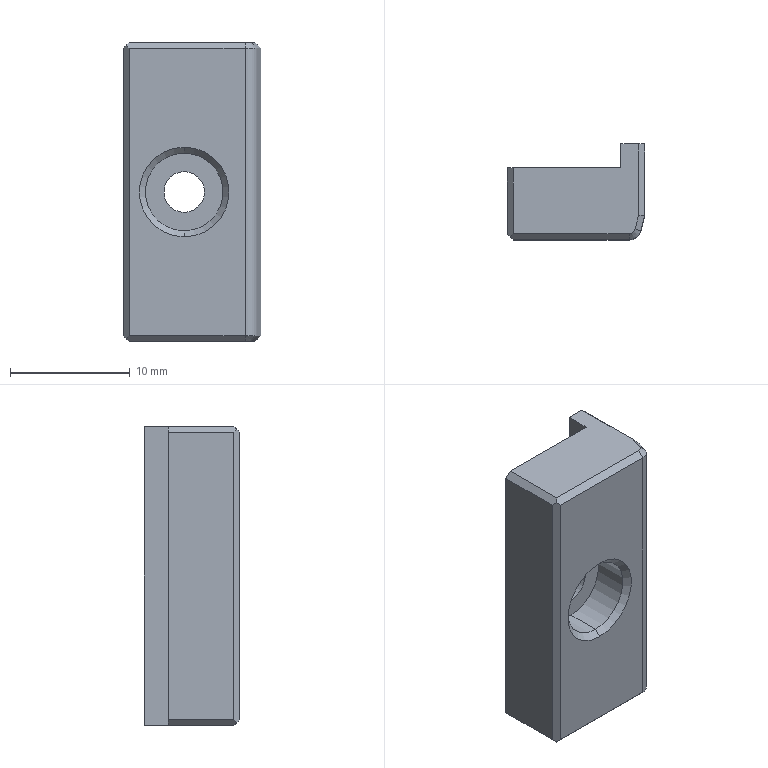Part | SolidWorks | features Chamfer 2, Extrusion 1, HoleWzd 1 | 1 solid | 28 faces | box 11.5 x 8 x 25 mm | volume 1661 mm3 | plane 19 | cylinder 5 | cone 4 | commonest cylinder face diameters 3.4 x2 6.5 x2 2 x1
STEP:
#1=CARTESIAN_POINT('',(-0.65,0.5,91.05));
#2=VERTEX_POINT('',#1);
#3=CARTESIAN_POINT('',(-0.65,0.5,84.55));
#4=VERTEX_POINT('',#3);
#5=CARTESIAN_POINT('',(-0.65,0.5,87.8));
#6=DIRECTION('',(0.,-1.,0.));
#7=DIRECTION('',(0.,0.,-1.));
#8=AXIS2_PLACEMENT_3D('',#5,#6,#7);
#9=CIRCLE('',#8,3.25);
#10=EDGE_CURVE('',#2,#4,#9,.T.);
#11=ORIENTED_EDGE('',*,*,#10,.F.);
#12=CARTESIAN_POINT('',(-0.65,0.,91.55));
#13=VERTEX_POINT('',#12);
#14=CARTESIAN_POINT('',(-0.65,0.5,91.05));
#15=DIRECTION('',(0.,-0.7071,0.7071));
#16=VECTOR('',#15,1000.);
#17=LINE('',#14,#16);
#18=EDGE_CURVE('',#2,#13,#17,.T.);
#19=ORIENTED_EDGE('',*,*,#18,.T.);
#20=CARTESIAN_POINT('',(-0.65,0.,84.05));
#21=VERTEX_POINT('',#20);
#22=CARTESIAN_POINT('',(-0.65,0.,87.8));
#23=DIRECTION('',(0.,1.,0.));
#24=DIRECTION('',(1.,0.,0.));
#25=AXIS2_PLACEMENT_3D('',#22,#23,#24);
#26=CIRCLE('',#25,3.75);
#27=EDGE_CURVE('',#21,#13,#26,.T.);
#28=ORIENTED_EDGE('',*,*,#27,.F.);
#29=CARTESIAN_POINT('',(-0.65,0.5,84.55));
#30=DIRECTION('',(0.,-0.7071,-0.7071));
#31=VECTOR('',#30,1000.);
#32=LINE('',#29,#31);
#33=EDGE_CURVE('',#4,#21,#32,.T.);
#34=ORIENTED_EDGE('',*,*,#33,.F.);
#35=EDGE_LOOP('',(#11,#19,#28,#34));
#36=FACE_OUTER_BOUND('',#35,.T.);
#37=CARTESIAN_POINT('',(-0.65,0.5,87.8));
#38=DIRECTION('',(0.,-1.,0.));
#39=DIRECTION('',(0.,0.,-1.));
#40=AXIS2_PLACEMENT_3D('',#37,#38,#39);
#41=CONICAL_SURFACE('',#40,3.25,0.7854);
#42=ADVANCED_FACE('',(#36),#41,.F.);
#43=CARTESIAN_POINT('',(-0.65,3.4,91.05));
#44=VERTEX_POINT('',#43);
#45=CARTESIAN_POINT('',(-0.65,3.4,84.55));
#46=VERTEX_POINT('',#45);
#47=CARTESIAN_POINT('',(-0.65,3.4,87.8));
#48=DIRECTION('',(0.,-1.,0.));
#49=DIRECTION('',(0.,0.,-1.));
#50=AXIS2_PLACEMENT_3D('',#47,#48,#49);
#51=CIRCLE('',#50,3.25);
#52=EDGE_CURVE('',#44,#46,#51,.T.);
#53=ORIENTED_EDGE('',*,*,#52,.F.);
#54=CARTESIAN_POINT('',(-0.65,0.,91.05));
#55=DIRECTION('',(0.,-1.,0.));
#56=VECTOR('',#55,1000.);
#57=LINE('',#54,#56);
#58=EDGE_CURVE('',#44,#2,#57,.T.);
#59=ORIENTED_EDGE('',*,*,#58,.T.);
#60=ORIENTED_EDGE('',*,*,#10,.T.);
#61=CARTESIAN_POINT('',(-0.65,0.,84.55));
#62=DIRECTION('',(0.,-1.,0.));
#63=VECTOR('',#62,1000.);
#64=LINE('',#61,#63);
#65=EDGE_CURVE('',#46,#4,#64,.T.);
#66=ORIENTED_EDGE('',*,*,#65,.F.);
#67=EDGE_LOOP('',(#53,#59,#60,#66));
#68=FACE_OUTER_BOUND('',#67,.T.);
#69=CARTESIAN_POINT('',(-0.65,0.,87.8));
#70=DIRECTION('',(0.,-1.,0.));
#71=DIRECTION('',(0.,0.,-1.));
#72=AXIS2_PLACEMENT_3D('',#69,#70,#71);
#73=CYLINDRICAL_SURFACE('',#72,3.25);
#74=ADVANCED_FACE('',(#68),#73,.F.);
#75=CARTESIAN_POINT('',(-0.65,6.,86.1));
#76=VERTEX_POINT('',#75);
#77=CARTESIAN_POINT('',(-0.65,6.,89.5));
#78=VERTEX_POINT('',#77);
#79=CARTESIAN_POINT('',(-0.65,6.,87.8));
#80=DIRECTION('',(0.,1.,0.));
#81=DIRECTION('',(0.,0.,1.));
#82=AXIS2_PLACEMENT_3D('',#79,#80,#81);
#83=CIRCLE('',#82,1.7);
#84=EDGE_CURVE('',#76,#78,#83,.T.);
#85=ORIENTED_EDGE('',*,*,#84,.T.);
#86=CARTESIAN_POINT('',(-0.65,3.4,89.5));
#87=VERTEX_POINT('',#86);
#88=CARTESIAN_POINT('',(-0.65,0.,89.5));
#89=DIRECTION('',(0.,-1.,0.));
#90=VECTOR('',#89,1000.);
#91=LINE('',#88,#90);
#92=EDGE_CURVE('',#78,#87,#91,.T.);
#93=ORIENTED_EDGE('',*,*,#92,.T.);
#94=CARTESIAN_POINT('',(-0.65,3.4,86.1));
#95=VERTEX_POINT('',#94);
#96=CARTESIAN_POINT('',(-0.65,3.4,87.8));
#97=DIRECTION('',(0.,-1.,0.));
#98=DIRECTION('',(0.,0.,-1.));
#99=AXIS2_PLACEMENT_3D('',#96,#97,#98);
#100=CIRCLE('',#99,1.7);
#101=EDGE_CURVE('',#87,#95,#100,.T.);
#102=ORIENTED_EDGE('',*,*,#101,.T.);
#103=CARTESIAN_POINT('',(-0.65,0.,86.1));
#104=DIRECTION('',(0.,-1.,0.));
#105=VECTOR('',#104,1000.);
#106=LINE('',#103,#105);
#107=EDGE_CURVE('',#76,#95,#106,.T.);
#108=ORIENTED_EDGE('',*,*,#107,.F.);
#109=EDGE_LOOP('',(#85,#93,#102,#108));
#110=FACE_OUTER_BOUND('',#109,.T.);
#111=CARTESIAN_POINT('',(-0.65,0.,87.8));
#112=DIRECTION('',(0.,-1.,0.));
#113=DIRECTION('',(0.,0.,-1.));
#114=AXIS2_PLACEMENT_3D('',#111,#112,#113);
#115=CYLINDRICAL_SURFACE('',#114,1.7);
#116=ADVANCED_FACE('',(#110),#115,.F.);
#117=CARTESIAN_POINT('',(3.75,6.,75.3));
#118=VERTEX_POINT('',#117);
#119=CARTESIAN_POINT('',(3.75,8.,75.3));
#120=VERTEX_POINT('',#119);
#121=CARTESIAN_POINT('',(3.75,8.,75.3));
#122=DIRECTION('',(0.,1.,0.));
#123=VECTOR('',#122,1000.);
#124=LINE('',#121,#123);
#125=EDGE_CURVE('',#118,#120,#124,.T.);
#126=ORIENTED_EDGE('',*,*,#125,.F.);
#127=CARTESIAN_POINT('',(3.75,6.,100.3));
#128=VERTEX_POINT('',#127);
#129=CARTESIAN_POINT('',(3.75,6.,61.291));
#130=DIRECTION('',(0.,0.,1.));
#131=VECTOR('',#130,1000.);
#132=LINE('',#129,#131);
#133=EDGE_CURVE('',#118,#128,#132,.T.);
#134=ORIENTED_EDGE('',*,*,#133,.T.);
#135=CARTESIAN_POINT('',(3.75,8.,100.3));
#136=VERTEX_POINT('',#135);
#137=CARTESIAN_POINT('',(3.75,8.,100.3));
#138=DIRECTION('',(0.,-1.,0.));
#139=VECTOR('',#138,1000.);
#140=LINE('',#137,#139);
#141=EDGE_CURVE('',#136,#128,#140,.T.);
#142=ORIENTED_EDGE('',*,*,#141,.F.);
#143=CARTESIAN_POINT('',(3.75,8.,61.291));
#144=DIRECTION('',(0.,0.,1.));
#145=VECTOR('',#144,1000.);
#146=LINE('',#143,#145);
#147=EDGE_CURVE('',#120,#136,#146,.T.);
#148=ORIENTED_EDGE('',*,*,#147,.F.);
#149=EDGE_LOOP('',(#126,#134,#142,#148));
#150=FACE_OUTER_BOUND('',#149,.T.);
#151=CARTESIAN_POINT('',(3.75,8.,61.291));
#152=DIRECTION('',(-1.,0.,0.));
#153=DIRECTION('',(0.,0.,1.));
#154=AXIS2_PLACEMENT_3D('',#151,#152,#153);
#155=PLANE('',#154);
#156=ADVANCED_FACE('',(#150),#155,.T.);
#157=CARTESIAN_POINT('',(5.25,8.,100.3));
#158=VERTEX_POINT('',#157);
#159=CARTESIAN_POINT('',(3.75,8.,100.3));
#160=DIRECTION('',(-1.,0.,0.));
#161=VECTOR('',#160,1000.);
#162=LINE('',#159,#161);
#163=EDGE_CURVE('',#158,#136,#162,.T.);
#164=ORIENTED_EDGE('',*,*,#163,.F.);
#165=CARTESIAN_POINT('',(5.75,8.,99.8));
#166=VERTEX_POINT('',#165);
#167=CARTESIAN_POINT('',(24.004,8.,81.546));
#168=DIRECTION('',(0.7071,0.,-0.7071));
#169=VECTOR('',#168,1000.);
#170=LINE('',#167,#169);
#171=EDGE_CURVE('',#158,#166,#170,.T.);
#172=ORIENTED_EDGE('',*,*,#171,.T.);
#173=CARTESIAN_POINT('',(5.75,8.,75.8));
#174=VERTEX_POINT('',#173);
#175=CARTESIAN_POINT('',(5.75,8.,61.291));
#176=DIRECTION('',(0.,0.,1.));
#177=VECTOR('',#176,1000.);
#178=LINE('',#175,#177);
#179=EDGE_CURVE('',#174,#166,#178,.T.);
#180=ORIENTED_EDGE('',*,*,#179,.F.);
#181=CARTESIAN_POINT('',(5.25,8.,75.3));
#182=VERTEX_POINT('',#181);
#183=CARTESIAN_POINT('',(-2.504,8.,67.546));
#184=DIRECTION('',(-0.7071,0.,-0.7071));
#185=VECTOR('',#184,1000.);
#186=LINE('',#183,#185);
#187=EDGE_CURVE('',#174,#182,#186,.T.);
#188=ORIENTED_EDGE('',*,*,#187,.T.);
#189=CARTESIAN_POINT('',(3.75,8.,75.3));
#190=DIRECTION('',(1.,0.,0.));
#191=VECTOR('',#190,1000.);
#192=LINE('',#189,#191);
#193=EDGE_CURVE('',#120,#182,#192,.T.);
#194=ORIENTED_EDGE('',*,*,#193,.F.);
#195=ORIENTED_EDGE('',*,*,#147,.T.);
#196=EDGE_LOOP('',(#164,#172,#180,#188,#194,#195));
#197=FACE_OUTER_BOUND('',#196,.T.);
#198=CARTESIAN_POINT('',(3.75,8.,61.291));
#199=DIRECTION('',(0.,1.,0.));
#200=DIRECTION('',(0.,0.,1.));
#201=AXIS2_PLACEMENT_3D('',#198,#199,#200);
#202=PLANE('',#201);
#203=ADVANCED_FACE('',(#197),#202,.T.);
#204=ORIENTED_EDGE('',*,*,#179,.T.);
#205=CARTESIAN_POINT('',(5.75,2.,99.8));
#206=VERTEX_POINT('',#205);
#207=CARTESIAN_POINT('',(5.75,8.,99.8));
#208=DIRECTION('',(0.,-1.,0.));
#209=VECTOR('',#208,1000.);
#210=LINE('',#207,#209);
#211=EDGE_CURVE('',#166,#206,#210,.T.);
#212=ORIENTED_EDGE('',*,*,#211,.T.);
#213=CARTESIAN_POINT('',(5.75,2.,75.8));
#214=VERTEX_POINT('',#213);
#215=CARTESIAN_POINT('',(5.75,2.,61.291));
#216=DIRECTION('',(0.,0.,1.));
#217=VECTOR('',#216,1000.);
#218=LINE('',#215,#217);
#219=EDGE_CURVE('',#214,#206,#218,.T.);
#220=ORIENTED_EDGE('',*,*,#219,.F.);
#221=CARTESIAN_POINT('',(5.75,8.,75.8));
#222=DIRECTION('',(0.,1.,0.));
#223=VECTOR('',#222,1000.);
#224=LINE('',#221,#223);
#225=EDGE_CURVE('',#214,#174,#224,.T.);
#226=ORIENTED_EDGE('',*,*,#225,.T.);
#227=EDGE_LOOP('',(#204,#212,#220,#226));
#228=FACE_OUTER_BOUND('',#227,.T.);
#229=CARTESIAN_POINT('',(5.75,8.,61.291));
#230=DIRECTION('',(1.,0.,0.));
#231=DIRECTION('',(0.,0.,-1.));
#232=AXIS2_PLACEMENT_3D('',#229,#230,#231);
#233=PLANE('',#232);
#234=ADVANCED_FACE('',(#228),#233,.T.);
#235=ORIENTED_EDGE('',*,*,#219,.T.);
#236=CARTESIAN_POINT('',(5.413,0.7412,99.8));
#237=VERTEX_POINT('',#236);
#238=CARTESIAN_POINT('',(5.75,2.,99.8));
#239=DIRECTION('',(-0.2588,-0.9659,0.));
#240=VECTOR('',#239,1000.);
#241=LINE('',#238,#240);
#242=EDGE_CURVE('',#206,#237,#241,.T.);
#243=ORIENTED_EDGE('',*,*,#242,.T.);
#244=CARTESIAN_POINT('',(5.413,0.7412,75.8));
#245=VERTEX_POINT('',#244);
#246=CARTESIAN_POINT('',(5.413,0.7412,61.291));
#247=DIRECTION('',(0.,0.,1.));
#248=VECTOR('',#247,1000.);
#249=LINE('',#246,#248);
#250=EDGE_CURVE('',#245,#237,#249,.T.);
#251=ORIENTED_EDGE('',*,*,#250,.F.);
#252=CARTESIAN_POINT('',(5.75,2.,75.8));
#253=DIRECTION('',(0.2588,0.9659,0.));
#254=VECTOR('',#253,1000.);
#255=LINE('',#252,#254);
#256=EDGE_CURVE('',#245,#214,#255,.T.);
#257=ORIENTED_EDGE('',*,*,#256,.T.);
#258=EDGE_LOOP('',(#235,#243,#251,#257));
#259=FACE_OUTER_BOUND('',#258,.T.);
#260=CARTESIAN_POINT('',(5.75,2.,61.291));
#261=DIRECTION('',(0.9659,-0.2588,0.));
#262=DIRECTION('',(0.2588,0.9659,0.));
#263=AXIS2_PLACEMENT_3D('',#260,#261,#262);
#264=PLANE('',#263);
#265=ADVANCED_FACE('',(#259),#264,.T.);
#266=ORIENTED_EDGE('',*,*,#250,.T.);
#267=CARTESIAN_POINT('',(4.447,0.,99.8));
#268=VERTEX_POINT('',#267);
#269=CARTESIAN_POINT('',(4.447,1.,99.8));
#270=DIRECTION('',(0.,0.,-1.));
#271=DIRECTION('',(1.,0.,0.));
#272=AXIS2_PLACEMENT_3D('',#269,#270,#271);
#273=CIRCLE('',#272,1.);
#274=EDGE_CURVE('',#237,#268,#273,.T.);
#275=ORIENTED_EDGE('',*,*,#274,.T.);
#276=CARTESIAN_POINT('',(4.447,0.,75.8));
#277=VERTEX_POINT('',#276);
#278=CARTESIAN_POINT('',(4.447,0.,61.291));
#279=DIRECTION('',(0.,0.,1.));
#280=VECTOR('',#279,1000.);
#281=LINE('',#278,#280);
#282=EDGE_CURVE('',#277,#268,#281,.T.);
#283=ORIENTED_EDGE('',*,*,#282,.F.);
#284=CARTESIAN_POINT('',(4.447,1.,75.8));
#285=DIRECTION('',(0.,0.,1.));
#286=DIRECTION('',(1.,0.,0.));
#287=AXIS2_PLACEMENT_3D('',#284,#285,#286);
#288=CIRCLE('',#287,1.);
#289=EDGE_CURVE('',#277,#245,#288,.T.);
#290=ORIENTED_EDGE('',*,*,#289,.T.);
#291=EDGE_LOOP('',(#266,#275,#283,#290));
#292=FACE_OUTER_BOUND('',#291,.T.);
#293=CARTESIAN_POINT('',(4.447,1.,61.291));
#294=DIRECTION('',(0.,0.,1.));
#295=DIRECTION('',(1.,0.,0.));
#296=AXIS2_PLACEMENT_3D('',#293,#294,#295);
#297=CYLINDRICAL_SURFACE('',#296,1.);
#298=ADVANCED_FACE('',(#292),#297,.T.);
#299=ORIENTED_EDGE('',*,*,#27,.T.);
#300=CARTESIAN_POINT('',(-0.65,0.,87.8));
#301=DIRECTION('',(0.,1.,0.));
#302=DIRECTION('',(1.,0.,0.));
#303=AXIS2_PLACEMENT_3D('',#300,#301,#302);
#304=CIRCLE('',#303,3.75);
#305=EDGE_CURVE('',#13,#21,#304,.T.);
#306=ORIENTED_EDGE('',*,*,#305,.T.);
#307=EDGE_LOOP('',(#299,#306));
#308=FACE_BOUND('',#307,.T.);
#309=ORIENTED_EDGE('',*,*,#282,.T.);
#310=CARTESIAN_POINT('',(-5.25,0.,99.8));
#311=VERTEX_POINT('',#310);
#312=CARTESIAN_POINT('',(4.447,0.,99.8));
#313=DIRECTION('',(-1.,0.,0.));
#314=VECTOR('',#313,1000.);
#315=LINE('',#312,#314);
#316=EDGE_CURVE('',#268,#311,#315,.T.);
#317=ORIENTED_EDGE('',*,*,#316,.T.);
#318=CARTESIAN_POINT('',(-5.25,0.,75.8));
#319=VERTEX_POINT('',#318);
#320=CARTESIAN_POINT('',(-5.25,0.,61.291));
#321=DIRECTION('',(0.,0.,1.));
#322=VECTOR('',#321,1000.);
#323=LINE('',#320,#322);
#324=EDGE_CURVE('',#319,#311,#323,.T.);
#325=ORIENTED_EDGE('',*,*,#324,.F.);
#326=CARTESIAN_POINT('',(4.447,0.,75.8));
#327=DIRECTION('',(1.,0.,0.));
#328=VECTOR('',#327,1000.);
#329=LINE('',#326,#328);
#330=EDGE_CURVE('',#319,#277,#329,.T.);
#331=ORIENTED_EDGE('',*,*,#330,.T.);
#332=EDGE_LOOP('',(#309,#317,#325,#331));
#333=FACE_OUTER_BOUND('',#332,.T.);
#334=CARTESIAN_POINT('',(4.447,0.,61.291));
#335=DIRECTION('',(0.,-1.,0.));
#336=DIRECTION('',(1.,0.,0.));
#337=AXIS2_PLACEMENT_3D('',#334,#335,#336);
#338=PLANE('',#337);
#339=ADVANCED_FACE('',(#308,#333),#338,.T.);
#340=CARTESIAN_POINT('',(-5.75,0.5,75.8));
#341=VERTEX_POINT('',#340);
#342=CARTESIAN_POINT('',(-5.5,0.25,75.55));
#343=VERTEX_POINT('',#342);
#344=CARTESIAN_POINT('',(-0.5804,-4.67,70.63));
#345=DIRECTION('',(0.5774,-0.5774,-0.5774));
#346=VECTOR('',#345,1000.);
#347=LINE('',#344,#346);
#348=EDGE_CURVE('',#341,#343,#347,.T.);
#349=ORIENTED_EDGE('',*,*,#348,.T.);
#350=CARTESIAN_POINT('',(-10.086,4.836,70.964));
#351=DIRECTION('',(0.5774,-0.5774,0.5774));
#352=VECTOR('',#351,1000.);
#353=LINE('',#350,#352);
#354=EDGE_CURVE('',#343,#319,#353,.T.);
#355=ORIENTED_EDGE('',*,*,#354,.T.);
#356=ORIENTED_EDGE('',*,*,#324,.T.);
#357=CARTESIAN_POINT('',(-5.5,0.25,100.05));
#358=VERTEX_POINT('',#357);
#359=CARTESIAN_POINT('',(7.586,-12.836,86.964));
#360=DIRECTION('',(-0.5774,0.5774,0.5774));
#361=VECTOR('',#360,1000.);
#362=LINE('',#359,#361);
#363=EDGE_CURVE('',#311,#358,#362,.T.);
#364=ORIENTED_EDGE('',*,*,#363,.T.);
#365=CARTESIAN_POINT('',(-5.75,0.5,99.8));
#366=VERTEX_POINT('',#365);
#367=CARTESIAN_POINT('',(-18.253,13.003,87.297));
#368=DIRECTION('',(-0.5774,0.5774,-0.5774));
#369=VECTOR('',#368,1000.);
#370=LINE('',#367,#369);
#371=EDGE_CURVE('',#358,#366,#370,.T.);
#372=ORIENTED_EDGE('',*,*,#371,.T.);
#373=CARTESIAN_POINT('',(-5.75,0.5,61.291));
#374=DIRECTION('',(0.,0.,1.));
#375=VECTOR('',#374,1000.);
#376=LINE('',#373,#375);
#377=EDGE_CURVE('',#341,#366,#376,.T.);
#378=ORIENTED_EDGE('',*,*,#377,.F.);
#379=EDGE_LOOP('',(#349,#355,#356,#364,#372,#378));
#380=FACE_OUTER_BOUND('',#379,.T.);
#381=CARTESIAN_POINT('',(-5.25,0.,61.291));
#382=DIRECTION('',(-0.7071,-0.7071,0.));
#383=DIRECTION('',(0.7071,-0.7071,0.));
#384=AXIS2_PLACEMENT_3D('',#381,#382,#383);
#385=PLANE('',#384);
#386=ADVANCED_FACE('',(#380),#385,.T.);
#387=CARTESIAN_POINT('',(-5.75,6.,75.8));
#388=VERTEX_POINT('',#387);
#389=CARTESIAN_POINT('',(-5.75,6.,99.8));
#390=VERTEX_POINT('',#389);
#391=CARTESIAN_POINT('',(-5.75,6.,61.291));
#392=DIRECTION('',(0.,0.,1.));
#393=VECTOR('',#392,1000.);
#394=LINE('',#391,#393);
#395=EDGE_CURVE('',#388,#390,#394,.T.);
#396=ORIENTED_EDGE('',*,*,#395,.F.);
#397=CARTESIAN_POINT('',(-5.75,0.5,75.8));
#398=DIRECTION('',(0.,-1.,0.));
#399=VECTOR('',#398,1000.);
#400=LINE('',#397,#399);
#401=EDGE_CURVE('',#388,#341,#400,.T.);
#402=ORIENTED_EDGE('',*,*,#401,.T.);
#403=ORIENTED_EDGE('',*,*,#377,.T.);
#404=CARTESIAN_POINT('',(-5.75,0.5,99.8));
#405=DIRECTION('',(0.,1.,0.));
#406=VECTOR('',#405,1000.);
#407=LINE('',#404,#406);
#408=EDGE_CURVE('',#366,#390,#407,.T.);
#409=ORIENTED_EDGE('',*,*,#408,.T.);
#410=EDGE_LOOP('',(#396,#402,#403,#409));
#411=FACE_OUTER_BOUND('',#410,.T.);
#412=CARTESIAN_POINT('',(-5.75,0.5,61.291));
#413=DIRECTION('',(-1.,0.,0.));
#414=DIRECTION('',(0.,0.,1.));
#415=AXIS2_PLACEMENT_3D('',#412,#413,#414);
#416=PLANE('',#415);
#417=ADVANCED_FACE('',(#411),#416,.T.);
#418=ORIENTED_EDGE('',*,*,#84,.F.);
#419=CARTESIAN_POINT('',(-0.65,6.,87.8));
#420=DIRECTION('',(0.,1.,0.));
#421=DIRECTION('',(0.,0.,1.));
#422=AXIS2_PLACEMENT_3D('',#419,#420,#421);
#423=CIRCLE('',#422,1.7);
#424=EDGE_CURVE('',#78,#76,#423,.T.);
#425=ORIENTED_EDGE('',*,*,#424,.F.);
#426=EDGE_LOOP('',(#418,#425));
#427=FACE_BOUND('',#426,.T.);
#428=CARTESIAN_POINT('',(-5.25,6.,75.3));
#429=VERTEX_POINT('',#428);
#430=CARTESIAN_POINT('',(-5.75,6.,75.3));
#431=DIRECTION('',(1.,0.,0.));
#432=VECTOR('',#431,1000.);
#433=LINE('',#430,#432);
#434=EDGE_CURVE('',#429,#118,#433,.T.);
#435=ORIENTED_EDGE('',*,*,#434,.F.);
#436=CARTESIAN_POINT('',(1.504,6.,68.546));
#437=DIRECTION('',(-0.7071,0.,0.7071));
#438=VECTOR('',#437,1000.);
#439=LINE('',#436,#438);
#440=EDGE_CURVE('',#429,#388,#439,.T.);
#441=ORIENTED_EDGE('',*,*,#440,.T.);
#442=ORIENTED_EDGE('',*,*,#395,.T.);
#443=CARTESIAN_POINT('',(-5.25,6.,100.3));
#444=VERTEX_POINT('',#443);
#445=CARTESIAN_POINT('',(-25.004,6.,80.546));
#446=DIRECTION('',(0.7071,0.,0.7071));
#447=VECTOR('',#446,1000.);
#448=LINE('',#445,#447);
#449=EDGE_CURVE('',#390,#444,#448,.T.);
#450=ORIENTED_EDGE('',*,*,#449,.T.);
#451=CARTESIAN_POINT('',(-5.75,6.,100.3));
#452=DIRECTION('',(-1.,0.,0.));
#453=VECTOR('',#452,1000.);
#454=LINE('',#451,#453);
#455=EDGE_CURVE('',#128,#444,#454,.T.);
#456=ORIENTED_EDGE('',*,*,#455,.F.);
#457=ORIENTED_EDGE('',*,*,#133,.F.);
#458=EDGE_LOOP('',(#435,#441,#442,#450,#456,#457));
#459=FACE_OUTER_BOUND('',#458,.T.);
#460=CARTESIAN_POINT('',(-5.75,6.,61.291));
#461=DIRECTION('',(0.,1.,0.));
#462=DIRECTION('',(0.,0.,1.));
#463=AXIS2_PLACEMENT_3D('',#460,#461,#462);
#464=PLANE('',#463);
#465=ADVANCED_FACE('',(#427,#459),#464,.T.);
#466=CARTESIAN_POINT('',(4.93,0.8706,100.3));
#467=VERTEX_POINT('',#466);
#468=CARTESIAN_POINT('',(5.25,2.066,100.3));
#469=VERTEX_POINT('',#468);
#470=CARTESIAN_POINT('',(4.93,0.8706,100.3));
#471=DIRECTION('',(0.2588,0.9659,0.));
#472=VECTOR('',#471,1000.);
#473=LINE('',#470,#472);
#474=EDGE_CURVE('',#467,#469,#473,.T.);
#475=ORIENTED_EDGE('',*,*,#474,.T.);
#476=CARTESIAN_POINT('',(5.25,1.,100.3));
#477=DIRECTION('',(0.,1.,0.));
#478=VECTOR('',#477,1000.);
#479=LINE('',#476,#478);
#480=EDGE_CURVE('',#469,#158,#479,.T.);
#481=ORIENTED_EDGE('',*,*,#480,.T.);
#482=ORIENTED_EDGE('',*,*,#163,.T.);
#483=ORIENTED_EDGE('',*,*,#141,.T.);
#484=ORIENTED_EDGE('',*,*,#455,.T.);
#485=CARTESIAN_POINT('',(-5.25,0.5,100.3));
#486=VERTEX_POINT('',#485);
#487=CARTESIAN_POINT('',(-5.25,1.,100.3));
#488=DIRECTION('',(0.,-1.,0.));
#489=VECTOR('',#488,1000.);
#490=LINE('',#487,#489);
#491=EDGE_CURVE('',#444,#486,#490,.T.);
#492=ORIENTED_EDGE('',*,*,#491,.T.);
#493=CARTESIAN_POINT('',(4.447,0.5,100.3));
#494=VERTEX_POINT('',#493);
#495=CARTESIAN_POINT('',(4.447,0.5,100.3));
#496=DIRECTION('',(1.,0.,0.));
#497=VECTOR('',#496,1000.);
#498=LINE('',#495,#497);
#499=EDGE_CURVE('',#486,#494,#498,.T.);
#500=ORIENTED_EDGE('',*,*,#499,.T.);
#501=CARTESIAN_POINT('',(4.447,1.,100.3));
#502=DIRECTION('',(0.,0.,1.));
#503=DIRECTION('',(1.,0.,0.));
#504=AXIS2_PLACEMENT_3D('',#501,#502,#503);
#505=CIRCLE('',#504,0.5);
#506=EDGE_CURVE('',#494,#467,#505,.T.);
#507=ORIENTED_EDGE('',*,*,#506,.T.);
#508=EDGE_LOOP('',(#475,#481,#482,#483,#484,#492,#500,#507));
#509=FACE_OUTER_BOUND('',#508,.T.);
#510=CARTESIAN_POINT('',(4.447,1.,100.3));
#511=DIRECTION('',(0.,0.,1.));
#512=DIRECTION('',(1.,0.,0.));
#513=AXIS2_PLACEMENT_3D('',#510,#511,#512);
#514=PLANE('',#513);
#515=ADVANCED_FACE('',(#509),#514,.T.);
#516=CARTESIAN_POINT('',(4.447,0.5,75.3));
#517=VERTEX_POINT('',#516);
#518=CARTESIAN_POINT('',(-5.25,0.5,75.3));
#519=VERTEX_POINT('',#518);
#520=CARTESIAN_POINT('',(-5.25,0.5,75.3));
#521=DIRECTION('',(-1.,0.,0.));
#522=VECTOR('',#521,1000.);
#523=LINE('',#520,#522);
#524=EDGE_CURVE('',#517,#519,#523,.T.);
#525=ORIENTED_EDGE('',*,*,#524,.T.);
#526=CARTESIAN_POINT('',(-5.25,6.,75.3));
#527=DIRECTION('',(0.,1.,0.));
#528=VECTOR('',#527,1000.);
#529=LINE('',#526,#528);
#530=EDGE_CURVE('',#519,#429,#529,.T.);
#531=ORIENTED_EDGE('',*,*,#530,.T.);
#532=ORIENTED_EDGE('',*,*,#434,.T.);
#533=ORIENTED_EDGE('',*,*,#125,.T.);
#534=ORIENTED_EDGE('',*,*,#193,.T.);
#535=CARTESIAN_POINT('',(5.25,2.066,75.3));
#536=VERTEX_POINT('',#535);
#537=CARTESIAN_POINT('',(5.25,2.,75.3));
#538=DIRECTION('',(0.,-1.,0.));
#539=VECTOR('',#538,1000.);
#540=LINE('',#537,#539);
#541=EDGE_CURVE('',#182,#536,#540,.T.);
#542=ORIENTED_EDGE('',*,*,#541,.T.);
#543=CARTESIAN_POINT('',(4.93,0.8706,75.3));
#544=VERTEX_POINT('',#543);
#545=CARTESIAN_POINT('',(4.93,0.8706,75.3));
#546=DIRECTION('',(-0.2588,-0.9659,0.));
#547=VECTOR('',#546,1000.);
#548=LINE('',#545,#547);
#549=EDGE_CURVE('',#536,#544,#548,.T.);
#550=ORIENTED_EDGE('',*,*,#549,.T.);
#551=CARTESIAN_POINT('',(4.447,1.,75.3));
#552=DIRECTION('',(0.,0.,-1.));
#553=DIRECTION('',(1.,0.,0.));
#554=AXIS2_PLACEMENT_3D('',#551,#552,#553);
#555=CIRCLE('',#554,0.5);
#556=EDGE_CURVE('',#544,#517,#555,.T.);
#557=ORIENTED_EDGE('',*,*,#556,.T.);
#558=EDGE_LOOP('',(#525,#531,#532,#533,#534,#542,#550,#557));
#559=FACE_OUTER_BOUND('',#558,.T.);
#560=CARTESIAN_POINT('',(5.75,6.,75.3));
#561=DIRECTION('',(0.,0.,1.));
#562=DIRECTION('',(1.,0.,0.));
#563=AXIS2_PLACEMENT_3D('',#560,#561,#562);
#564=PLANE('',#563);
#565=ADVANCED_FACE('',(#559),#564,.F.);
#566=ORIENTED_EDGE('',*,*,#408,.F.);
#567=ORIENTED_EDGE('',*,*,#371,.F.);
#568=CARTESIAN_POINT('',(-2.018,3.732,103.532));
#569=DIRECTION('',(-0.5774,-0.5774,-0.5774));
#570=VECTOR('',#569,1000.);
#571=LINE('',#568,#570);
#572=EDGE_CURVE('',#486,#358,#571,.T.);
#573=ORIENTED_EDGE('',*,*,#572,.F.);
#574=ORIENTED_EDGE('',*,*,#491,.F.);
#575=ORIENTED_EDGE('',*,*,#449,.F.);
#576=EDGE_LOOP('',(#566,#567,#573,#574,#575));
#577=FACE_OUTER_BOUND('',#576,.T.);
#578=CARTESIAN_POINT('',(-5.25,1.,100.3));
#579=DIRECTION('',(0.7071,0.,-0.7071));
#580=DIRECTION('',(0.,-1.,0.));
#581=AXIS2_PLACEMENT_3D('',#578,#579,#580);
#582=PLANE('',#581);
#583=ADVANCED_FACE('',(#577),#582,.F.);
#584=ORIENTED_EDGE('',*,*,#363,.F.);
#585=ORIENTED_EDGE('',*,*,#316,.F.);
#586=CARTESIAN_POINT('',(4.447,0.5,100.3));
#587=DIRECTION('',(0.,-0.7071,-0.7071));
#588=VECTOR('',#587,1000.);
#589=LINE('',#586,#588);
#590=EDGE_CURVE('',#494,#268,#589,.T.);
#591=ORIENTED_EDGE('',*,*,#590,.F.);
#592=ORIENTED_EDGE('',*,*,#499,.F.);
#593=ORIENTED_EDGE('',*,*,#572,.T.);
#594=EDGE_LOOP('',(#584,#585,#591,#592,#593));
#595=FACE_OUTER_BOUND('',#594,.T.);
#596=CARTESIAN_POINT('',(4.447,0.5,100.3));
#597=DIRECTION('',(0.,0.7071,-0.7071));
#598=DIRECTION('',(1.,0.,0.));
#599=AXIS2_PLACEMENT_3D('',#596,#597,#598);
#600=PLANE('',#599);
#601=ADVANCED_FACE('',(#595),#600,.F.);
#602=ORIENTED_EDGE('',*,*,#590,.T.);
#603=ORIENTED_EDGE('',*,*,#274,.F.);
#604=CARTESIAN_POINT('',(4.93,0.8706,100.3));
#605=DIRECTION('',(0.683,-0.183,-0.7071));
#606=VECTOR('',#605,1000.);
#607=LINE('',#604,#606);
#608=EDGE_CURVE('',#467,#237,#607,.T.);
#609=ORIENTED_EDGE('',*,*,#608,.F.);
#610=ORIENTED_EDGE('',*,*,#506,.F.);
#611=EDGE_LOOP('',(#602,#603,#609,#610));
#612=FACE_OUTER_BOUND('',#611,.T.);
#613=CARTESIAN_POINT('',(4.447,1.,100.3));
#614=DIRECTION('',(0.,0.,-1.));
#615=DIRECTION('',(-1.,0.,0.));
#616=AXIS2_PLACEMENT_3D('',#613,#614,#615);
#617=CONICAL_SURFACE('',#616,0.5,0.7854);
#618=ADVANCED_FACE('',(#612),#617,.T.);
#619=ORIENTED_EDGE('',*,*,#608,.T.);
#620=ORIENTED_EDGE('',*,*,#242,.F.);
#621=CARTESIAN_POINT('',(5.169,2.076,100.381));
#622=DIRECTION('',(0.7041,-0.09269,-0.7041));
#623=VECTOR('',#622,1000.);
#624=LINE('',#621,#623);
#625=EDGE_CURVE('',#469,#206,#624,.T.);
#626=ORIENTED_EDGE('',*,*,#625,.F.);
#627=ORIENTED_EDGE('',*,*,#474,.F.);
#628=EDGE_LOOP('',(#619,#620,#626,#627));
#629=FACE_OUTER_BOUND('',#628,.T.);
#630=CARTESIAN_POINT('',(4.93,0.8706,100.3));
#631=DIRECTION('',(-0.683,0.183,-0.7071));
#632=DIRECTION('',(0.2588,0.9659,0.));
#633=AXIS2_PLACEMENT_3D('',#630,#631,#632);
#634=PLANE('',#633);
#635=ADVANCED_FACE('',(#629),#634,.F.);
#636=ORIENTED_EDGE('',*,*,#625,.T.);
#637=ORIENTED_EDGE('',*,*,#211,.F.);
#638=ORIENTED_EDGE('',*,*,#171,.F.);
#639=ORIENTED_EDGE('',*,*,#480,.F.);
#640=EDGE_LOOP('',(#636,#637,#638,#639));
#641=FACE_OUTER_BOUND('',#640,.T.);
#642=CARTESIAN_POINT('',(5.25,1.,100.3));
#643=DIRECTION('',(-0.7071,0.,-0.7071));
#644=DIRECTION('',(0.,1.,0.));
#645=AXIS2_PLACEMENT_3D('',#642,#643,#644);
#646=PLANE('',#645);
#647=ADVANCED_FACE('',(#641),#646,.F.);
#648=ORIENTED_EDGE('',*,*,#440,.F.);
#649=ORIENTED_EDGE('',*,*,#530,.F.);
#650=CARTESIAN_POINT('',(-3.417,2.333,73.467));
#651=DIRECTION('',(0.5774,0.5774,-0.5774));
#652=VECTOR('',#651,1000.);
#653=LINE('',#650,#652);
#654=EDGE_CURVE('',#343,#519,#653,.T.);
#655=ORIENTED_EDGE('',*,*,#654,.F.);
#656=ORIENTED_EDGE('',*,*,#348,.F.);
#657=ORIENTED_EDGE('',*,*,#401,.F.);
#658=EDGE_LOOP('',(#648,#649,#655,#656,#657));
#659=FACE_OUTER_BOUND('',#658,.T.);
#660=CARTESIAN_POINT('',(-5.25,6.,75.3));
#661=DIRECTION('',(-0.7071,0.,-0.7071));
#662=DIRECTION('',(0.,-1.,0.));
#663=AXIS2_PLACEMENT_3D('',#660,#661,#662);
#664=PLANE('',#663);
#665=ADVANCED_FACE('',(#659),#664,.T.);
#666=ORIENTED_EDGE('',*,*,#654,.T.);
#667=ORIENTED_EDGE('',*,*,#524,.F.);
#668=CARTESIAN_POINT('',(4.447,0.,75.8));
#669=DIRECTION('',(0.,0.7071,-0.7071));
#670=VECTOR('',#669,1000.);
#671=LINE('',#668,#670);
#672=EDGE_CURVE('',#277,#517,#671,.T.);
#673=ORIENTED_EDGE('',*,*,#672,.F.);
#674=ORIENTED_EDGE('',*,*,#330,.F.);
#675=ORIENTED_EDGE('',*,*,#354,.F.);
#676=EDGE_LOOP('',(#666,#667,#673,#674,#675));
#677=FACE_OUTER_BOUND('',#676,.T.);
#678=CARTESIAN_POINT('',(5.75,0.5,75.3));
#679=DIRECTION('',(0.,-0.7071,-0.7071));
#680=DIRECTION('',(1.,0.,0.));
#681=AXIS2_PLACEMENT_3D('',#678,#679,#680);
#682=PLANE('',#681);
#683=ADVANCED_FACE('',(#677),#682,.T.);
#684=ORIENTED_EDGE('',*,*,#187,.F.);
#685=ORIENTED_EDGE('',*,*,#225,.F.);
#686=CARTESIAN_POINT('',(4.993,2.1,75.043));
#687=DIRECTION('',(0.7041,-0.09269,0.7041));
#688=VECTOR('',#687,1000.);
#689=LINE('',#686,#688);
#690=EDGE_CURVE('',#536,#214,#689,.T.);
#691=ORIENTED_EDGE('',*,*,#690,.F.);
#692=ORIENTED_EDGE('',*,*,#541,.F.);
#693=EDGE_LOOP('',(#684,#685,#691,#692));
#694=FACE_OUTER_BOUND('',#693,.T.);
#695=CARTESIAN_POINT('',(5.25,6.,75.3));
#696=DIRECTION('',(0.7071,0.,-0.7071));
#697=DIRECTION('',(0.,1.,0.));
#698=AXIS2_PLACEMENT_3D('',#695,#696,#697);
#699=PLANE('',#698);
#700=ADVANCED_FACE('',(#694),#699,.T.);
#701=ORIENTED_EDGE('',*,*,#672,.T.);
#702=ORIENTED_EDGE('',*,*,#556,.F.);
#703=CARTESIAN_POINT('',(5.413,0.7412,75.8));
#704=DIRECTION('',(-0.683,0.183,-0.7071));
#705=VECTOR('',#704,1000.);
#706=LINE('',#703,#705);
#707=EDGE_CURVE('',#245,#544,#706,.T.);
#708=ORIENTED_EDGE('',*,*,#707,.F.);
#709=ORIENTED_EDGE('',*,*,#289,.F.);
#710=EDGE_LOOP('',(#701,#702,#708,#709));
#711=FACE_OUTER_BOUND('',#710,.T.);
#712=CARTESIAN_POINT('',(4.447,1.,75.3));
#713=DIRECTION('',(0.,0.,1.));
#714=DIRECTION('',(1.,0.,0.));
#715=AXIS2_PLACEMENT_3D('',#712,#713,#714);
#716=CONICAL_SURFACE('',#715,0.5,0.7854);
#717=ADVANCED_FACE('',(#711),#716,.T.);
#718=ORIENTED_EDGE('',*,*,#690,.T.);
#719=ORIENTED_EDGE('',*,*,#256,.F.);
#720=ORIENTED_EDGE('',*,*,#707,.T.);
#721=ORIENTED_EDGE('',*,*,#549,.F.);
#722=EDGE_LOOP('',(#718,#719,#720,#721));
#723=FACE_OUTER_BOUND('',#722,.T.);
#724=CARTESIAN_POINT('',(6.267,5.861,75.3));
#725=DIRECTION('',(0.683,-0.183,-0.7071));
#726=DIRECTION('',(0.2588,0.9659,0.));
#727=AXIS2_PLACEMENT_3D('',#724,#725,#726);
#728=PLANE('',#727);
#729=ADVANCED_FACE('',(#723),#728,.T.);
#730=ORIENTED_EDGE('',*,*,#92,.F.);
#731=ORIENTED_EDGE('',*,*,#424,.T.);
#732=ORIENTED_EDGE('',*,*,#107,.T.);
#733=CARTESIAN_POINT('',(-0.65,3.4,87.8));
#734=DIRECTION('',(0.,-1.,0.));
#735=DIRECTION('',(0.,0.,-1.));
#736=AXIS2_PLACEMENT_3D('',#733,#734,#735);
#737=CIRCLE('',#736,1.7);
#738=EDGE_CURVE('',#95,#87,#737,.T.);
#739=ORIENTED_EDGE('',*,*,#738,.T.);
#740=EDGE_LOOP('',(#730,#731,#732,#739));
#741=FACE_OUTER_BOUND('',#740,.T.);
#742=CARTESIAN_POINT('',(-0.65,0.,87.8));
#743=DIRECTION('',(0.,-1.,0.));
#744=DIRECTION('',(0.,0.,-1.));
#745=AXIS2_PLACEMENT_3D('',#742,#743,#744);
#746=CYLINDRICAL_SURFACE('',#745,1.7);
#747=ADVANCED_FACE('',(#741),#746,.F.);
#748=ORIENTED_EDGE('',*,*,#738,.F.);
#749=ORIENTED_EDGE('',*,*,#101,.F.);
#750=EDGE_LOOP('',(#748,#749));
#751=FACE_BOUND('',#750,.T.);
#752=CARTESIAN_POINT('',(-0.65,3.4,87.8));
#753=DIRECTION('',(0.,-1.,0.));
#754=DIRECTION('',(0.,0.,-1.));
#755=AXIS2_PLACEMENT_3D('',#752,#753,#754);
#756=CIRCLE('',#755,3.25);
#757=EDGE_CURVE('',#46,#44,#756,.T.);
#758=ORIENTED_EDGE('',*,*,#757,.T.);
#759=ORIENTED_EDGE('',*,*,#52,.T.);
#760=EDGE_LOOP('',(#758,#759));
#761=FACE_OUTER_BOUND('',#760,.T.);
#762=CARTESIAN_POINT('',(1.05,3.4,87.8));
#763=DIRECTION('',(0.,1.,0.));
#764=DIRECTION('',(0.,0.,1.));
#765=AXIS2_PLACEMENT_3D('',#762,#763,#764);
#766=PLANE('',#765);
#767=ADVANCED_FACE('',(#751,#761),#766,.F.);
#768=ORIENTED_EDGE('',*,*,#58,.F.);
#769=ORIENTED_EDGE('',*,*,#757,.F.);
#770=ORIENTED_EDGE('',*,*,#65,.T.);
#771=CARTESIAN_POINT('',(-0.65,0.5,87.8));
#772=DIRECTION('',(0.,-1.,0.));
#773=DIRECTION('',(0.,0.,-1.));
#774=AXIS2_PLACEMENT_3D('',#771,#772,#773);
#775=CIRCLE('',#774,3.25);
#776=EDGE_CURVE('',#4,#2,#775,.T.);
#777=ORIENTED_EDGE('',*,*,#776,.T.);
#778=EDGE_LOOP('',(#768,#769,#770,#777));
#779=FACE_OUTER_BOUND('',#778,.T.);
#780=CARTESIAN_POINT('',(-0.65,0.,87.8));
#781=DIRECTION('',(0.,-1.,0.));
#782=DIRECTION('',(0.,0.,-1.));
#783=AXIS2_PLACEMENT_3D('',#780,#781,#782);
#784=CYLINDRICAL_SURFACE('',#783,3.25);
#785=ADVANCED_FACE('',(#779),#784,.F.);
#786=ORIENTED_EDGE('',*,*,#18,.F.);
#787=ORIENTED_EDGE('',*,*,#776,.F.);
#788=ORIENTED_EDGE('',*,*,#33,.T.);
#789=ORIENTED_EDGE('',*,*,#305,.F.);
#790=EDGE_LOOP('',(#786,#787,#788,#789));
#791=FACE_OUTER_BOUND('',#790,.T.);
#792=CARTESIAN_POINT('',(-0.65,0.5,87.8));
#793=DIRECTION('',(0.,-1.,0.));
#794=DIRECTION('',(0.,0.,-1.));
#795=AXIS2_PLACEMENT_3D('',#792,#793,#794);
#796=CONICAL_SURFACE('',#795,3.25,0.7854);
#797=ADVANCED_FACE('',(#791),#796,.F.);
#798=CLOSED_SHELL('',(#42,#74,#116,#156,#203,#234,#265,#298,#339,#386,#417,#465,#515,#565,#583,#601,#618,#635,#647,#665,#683,#700,#717,#729,#747,#767,#785,#797));
#799=MANIFOLD_SOLID_BREP('',#798);
#800=CARTESIAN_POINT('',(0.,0.,0.));
#801=DIRECTION('',(0.,0.,1.));
#802=DIRECTION('',(1.,0.,0.));
#803=AXIS2_PLACEMENT_3D('',#800,#801,#802);
#804=(LENGTH_UNIT()NAMED_UNIT(*)SI_UNIT(.MILLI.,.METRE.));
#805=UNCERTAINTY_MEASURE_WITH_UNIT(LENGTH_MEASURE(0.00001),#804,'','');
#806=(NAMED_UNIT(*)PLANE_ANGLE_UNIT()SI_UNIT($,.RADIAN.));
#807=(NAMED_UNIT(*)SI_UNIT($,.STERADIAN.)SOLID_ANGLE_UNIT());
#808=(GEOMETRIC_REPRESENTATION_CONTEXT(3)GLOBAL_UNCERTAINTY_ASSIGNED_CONTEXT((#805))GLOBAL_UNIT_ASSIGNED_CONTEXT((#804,#806,#807))REPRESENTATION_CONTEXT('',''));
#809=ADVANCED_BREP_SHAPE_REPRESENTATION('',(#799,#803),#808);